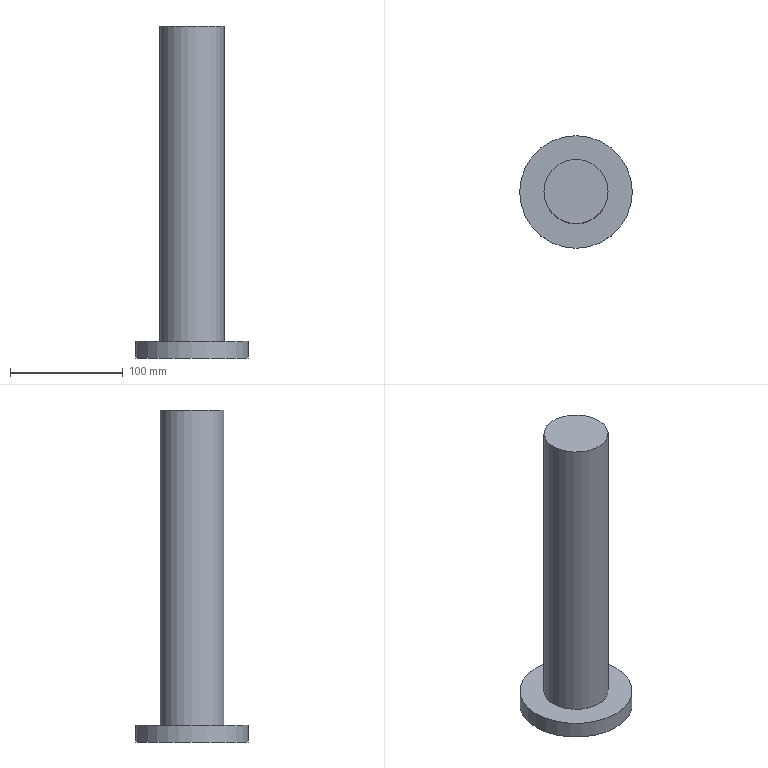Part | NX | features 立柱活塞销 2 | 1 solid | 5 faces | box 100 x 100 x 295 mm | volume 832302 mm3 | plane 3 | cylinder 2 | commonest cylinder face diameters 57 x1 100 x1
STEP:
#1=CARTESIAN_POINT('',(28.5,0.,280.));
#2=VERTEX_POINT('',#1);
#3=CARTESIAN_POINT('',(0.,0.,280.));
#4=DIRECTION('',(0.,0.,1.));
#5=DIRECTION('',(1.,0.,0.));
#6=AXIS2_PLACEMENT_3D('',#3,#4,#5);
#7=CIRCLE('',#6,28.5);
#8=EDGE_CURVE('',#2,#2,#7,.T.);
#9=ORIENTED_EDGE('',*,*,#8,.F.);
#10=EDGE_LOOP('',(#9));
#11=FACE_BOUND('',#10,.T.);
#12=CARTESIAN_POINT('',(-28.5,0.,0.));
#13=VERTEX_POINT('',#12);
#14=CARTESIAN_POINT('',(0.,0.,0.));
#15=DIRECTION('',(0.,0.,-1.));
#16=DIRECTION('',(-1.,0.,0.));
#17=AXIS2_PLACEMENT_3D('',#14,#15,#16);
#18=CIRCLE('',#17,28.5);
#19=EDGE_CURVE('',#13,#13,#18,.T.);
#20=ORIENTED_EDGE('',*,*,#19,.F.);
#21=EDGE_LOOP('',(#20));
#22=FACE_BOUND('',#21,.T.);
#23=CARTESIAN_POINT('',(0.,0.,280.));
#24=DIRECTION('',(0.,0.,-1.));
#25=DIRECTION('',(-1.,0.,0.));
#26=AXIS2_PLACEMENT_3D('',#23,#24,#25);
#27=CYLINDRICAL_SURFACE('',#26,28.5);
#28=ADVANCED_FACE('',(#11,#22),#27,.T.);
#29=ORIENTED_EDGE('',*,*,#8,.T.);
#30=EDGE_LOOP('',(#29));
#31=FACE_BOUND('',#30,.T.);
#32=CARTESIAN_POINT('',(0.,0.,280.));
#33=DIRECTION('',(0.,0.,1.));
#34=DIRECTION('',(1.,0.,0.));
#35=AXIS2_PLACEMENT_3D('',#32,#33,#34);
#36=PLANE('',#35);
#37=ADVANCED_FACE('',(#31),#36,.T.);
#38=CARTESIAN_POINT('',(-50.,0.,0.));
#39=VERTEX_POINT('',#38);
#40=CARTESIAN_POINT('',(0.,0.,0.));
#41=DIRECTION('',(0.,0.,-1.));
#42=DIRECTION('',(-1.,0.,0.));
#43=AXIS2_PLACEMENT_3D('',#40,#41,#42);
#44=CIRCLE('',#43,50.);
#45=EDGE_CURVE('',#39,#39,#44,.T.);
#46=ORIENTED_EDGE('',*,*,#45,.F.);
#47=EDGE_LOOP('',(#46));
#48=FACE_BOUND('',#47,.T.);
#49=ORIENTED_EDGE('',*,*,#19,.T.);
#50=EDGE_LOOP('',(#49));
#51=FACE_BOUND('',#50,.T.);
#52=CARTESIAN_POINT('',(0.,0.,0.));
#53=DIRECTION('',(0.,0.,-1.));
#54=DIRECTION('',(-1.,0.,0.));
#55=AXIS2_PLACEMENT_3D('',#52,#53,#54);
#56=PLANE('',#55);
#57=ADVANCED_FACE('',(#48,#51),#56,.F.);
#58=CARTESIAN_POINT('',(-50.,0.,-15.));
#59=VERTEX_POINT('',#58);
#60=CARTESIAN_POINT('',(0.,0.,-15.));
#61=DIRECTION('',(0.,0.,-1.));
#62=DIRECTION('',(-1.,0.,0.));
#63=AXIS2_PLACEMENT_3D('',#60,#61,#62);
#64=CIRCLE('',#63,50.);
#65=EDGE_CURVE('',#59,#59,#64,.T.);
#66=ORIENTED_EDGE('',*,*,#65,.F.);
#67=EDGE_LOOP('',(#66));
#68=FACE_BOUND('',#67,.T.);
#69=ORIENTED_EDGE('',*,*,#45,.T.);
#70=EDGE_LOOP('',(#69));
#71=FACE_BOUND('',#70,.T.);
#72=CARTESIAN_POINT('',(0.,0.,-15.));
#73=DIRECTION('',(0.,0.,1.));
#74=DIRECTION('',(1.,0.,0.));
#75=AXIS2_PLACEMENT_3D('',#72,#73,#74);
#76=CYLINDRICAL_SURFACE('',#75,50.);
#77=ADVANCED_FACE('',(#68,#71),#76,.T.);
#78=ORIENTED_EDGE('',*,*,#65,.T.);
#79=EDGE_LOOP('',(#78));
#80=FACE_BOUND('',#79,.T.);
#81=CARTESIAN_POINT('',(0.,0.,-15.));
#82=DIRECTION('',(0.,0.,-1.));
#83=DIRECTION('',(-1.,0.,0.));
#84=AXIS2_PLACEMENT_3D('',#81,#82,#83);
#85=PLANE('',#84);
#86=ADVANCED_FACE('',(#80),#85,.T.);
#87=CLOSED_SHELL('',(#28,#37,#57,#77,#86));
#88=MANIFOLD_SOLID_BREP('',#87);
#89=(LENGTH_UNIT()NAMED_UNIT(*)SI_UNIT(.MILLI.,.METRE.));
#90=UNCERTAINTY_MEASURE_WITH_UNIT(LENGTH_MEASURE(0.00001),#89,'','');
#91=(NAMED_UNIT(*)PLANE_ANGLE_UNIT()SI_UNIT($,.RADIAN.));
#92=(NAMED_UNIT(*)SI_UNIT($,.STERADIAN.)SOLID_ANGLE_UNIT());
#93=(GEOMETRIC_REPRESENTATION_CONTEXT(3)GLOBAL_UNCERTAINTY_ASSIGNED_CONTEXT((#90))GLOBAL_UNIT_ASSIGNED_CONTEXT((#89,#91,#92))REPRESENTATION_CONTEXT('',''));
#94=ADVANCED_BREP_SHAPE_REPRESENTATION('',(#88),#93);